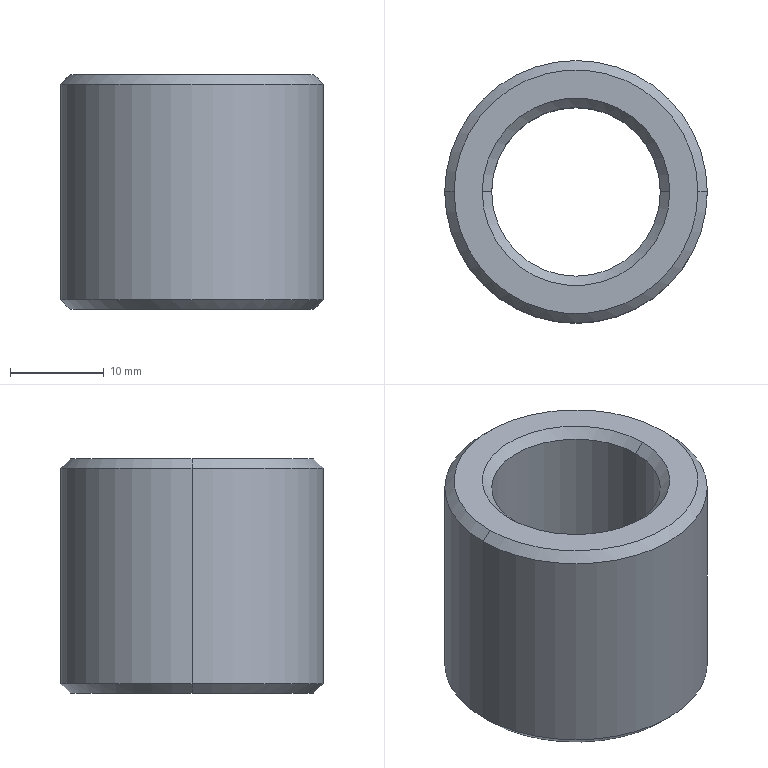Part | STEP file | VD-SYL0380DJ1006_1_2_1-9_2_STEP | 1 solid | 14 faces | box 28 x 28 x 25 mm | volume 8888 mm3 | cone 8 | cylinder 4 | plane 2 | commonest cylinder face diameters 18 x2 28 x2
STEP:
#1=CARTESIAN_POINT('',(9.,0.,-11.5));
#2=VERTEX_POINT('',#1);
#3=CARTESIAN_POINT('',(-9.,0.,-11.5));
#4=VERTEX_POINT('',#3);
#5=CARTESIAN_POINT('',(0.,0.,-11.5));
#6=DIRECTION('',(0.,0.,1.));
#7=DIRECTION('',(1.,0.,0.));
#8=AXIS2_PLACEMENT_3D('',#5,#6,#7);
#9=CIRCLE('',#8,9.);
#10=EDGE_CURVE('',#2,#4,#9,.T.);
#11=ORIENTED_EDGE('',*,*,#10,.F.);
#12=CARTESIAN_POINT('',(9.,0.,11.5));
#13=VERTEX_POINT('',#12);
#14=CARTESIAN_POINT('',(9.,0.,11.5));
#15=DIRECTION('',(0.,0.,-1.));
#16=VECTOR('',#15,1000.);
#17=LINE('',#14,#16);
#18=EDGE_CURVE('',#13,#2,#17,.T.);
#19=ORIENTED_EDGE('',*,*,#18,.F.);
#20=CARTESIAN_POINT('',(-9.,0.,11.5));
#21=VERTEX_POINT('',#20);
#22=CARTESIAN_POINT('',(0.,0.,11.5));
#23=DIRECTION('',(0.,0.,-1.));
#24=DIRECTION('',(-1.,0.,0.));
#25=AXIS2_PLACEMENT_3D('',#22,#23,#24);
#26=CIRCLE('',#25,9.);
#27=EDGE_CURVE('',#21,#13,#26,.T.);
#28=ORIENTED_EDGE('',*,*,#27,.F.);
#29=CARTESIAN_POINT('',(-9.,0.,11.5));
#30=DIRECTION('',(0.,0.,-1.));
#31=VECTOR('',#30,1000.);
#32=LINE('',#29,#31);
#33=EDGE_CURVE('',#21,#4,#32,.T.);
#34=ORIENTED_EDGE('',*,*,#33,.T.);
#35=EDGE_LOOP('',(#11,#19,#28,#34));
#36=FACE_OUTER_BOUND('',#35,.T.);
#37=CARTESIAN_POINT('',(0.,0.,-12.5));
#38=DIRECTION('',(0.,0.,1.));
#39=DIRECTION('',(1.,0.,0.));
#40=AXIS2_PLACEMENT_3D('',#37,#38,#39);
#41=CYLINDRICAL_SURFACE('',#40,9.);
#42=ADVANCED_FACE('',(#36),#41,.F.);
#43=ORIENTED_EDGE('',*,*,#27,.T.);
#44=CARTESIAN_POINT('',(10.,0.,12.5));
#45=VERTEX_POINT('',#44);
#46=CARTESIAN_POINT('',(10.,0.,12.5));
#47=DIRECTION('',(-0.7071,0.,-0.7071));
#48=VECTOR('',#47,1000.);
#49=LINE('',#46,#48);
#50=EDGE_CURVE('',#45,#13,#49,.T.);
#51=ORIENTED_EDGE('',*,*,#50,.F.);
#52=CARTESIAN_POINT('',(-10.,0.,12.5));
#53=VERTEX_POINT('',#52);
#54=CARTESIAN_POINT('',(0.,0.,12.5));
#55=DIRECTION('',(0.,0.,-1.));
#56=DIRECTION('',(-1.,0.,0.));
#57=AXIS2_PLACEMENT_3D('',#54,#55,#56);
#58=CIRCLE('',#57,10.);
#59=EDGE_CURVE('',#53,#45,#58,.T.);
#60=ORIENTED_EDGE('',*,*,#59,.F.);
#61=CARTESIAN_POINT('',(-10.,0.,12.5));
#62=DIRECTION('',(0.7071,0.,-0.7071));
#63=VECTOR('',#62,1000.);
#64=LINE('',#61,#63);
#65=EDGE_CURVE('',#53,#21,#64,.T.);
#66=ORIENTED_EDGE('',*,*,#65,.T.);
#67=EDGE_LOOP('',(#43,#51,#60,#66));
#68=FACE_OUTER_BOUND('',#67,.T.);
#69=CARTESIAN_POINT('',(0.,0.,12.));
#70=DIRECTION('',(0.,0.,1.));
#71=DIRECTION('',(1.,0.,0.));
#72=AXIS2_PLACEMENT_3D('',#69,#70,#71);
#73=CONICAL_SURFACE('',#72,9.5,0.7854);
#74=ADVANCED_FACE('',(#68),#73,.F.);
#75=ORIENTED_EDGE('',*,*,#65,.F.);
#76=CARTESIAN_POINT('',(0.,0.,12.5));
#77=DIRECTION('',(0.,0.,-1.));
#78=DIRECTION('',(1.,0.,0.));
#79=AXIS2_PLACEMENT_3D('',#76,#77,#78);
#80=CIRCLE('',#79,10.);
#81=EDGE_CURVE('',#45,#53,#80,.T.);
#82=ORIENTED_EDGE('',*,*,#81,.F.);
#83=ORIENTED_EDGE('',*,*,#50,.T.);
#84=CARTESIAN_POINT('',(0.,0.,11.5));
#85=DIRECTION('',(0.,0.,-1.));
#86=DIRECTION('',(1.,0.,0.));
#87=AXIS2_PLACEMENT_3D('',#84,#85,#86);
#88=CIRCLE('',#87,9.);
#89=EDGE_CURVE('',#13,#21,#88,.T.);
#90=ORIENTED_EDGE('',*,*,#89,.T.);
#91=EDGE_LOOP('',(#75,#82,#83,#90));
#92=FACE_OUTER_BOUND('',#91,.T.);
#93=CARTESIAN_POINT('',(0.,0.,12.));
#94=DIRECTION('',(0.,0.,1.));
#95=DIRECTION('',(1.,0.,0.));
#96=AXIS2_PLACEMENT_3D('',#93,#94,#95);
#97=CONICAL_SURFACE('',#96,9.5,0.7854);
#98=ADVANCED_FACE('',(#92),#97,.F.);
#99=CARTESIAN_POINT('',(-13.,0.,12.5));
#100=VERTEX_POINT('',#99);
#101=CARTESIAN_POINT('',(13.,0.,12.5));
#102=VERTEX_POINT('',#101);
#103=CARTESIAN_POINT('',(0.,0.,12.5));
#104=DIRECTION('',(0.,0.,1.));
#105=DIRECTION('',(-1.,0.,0.));
#106=AXIS2_PLACEMENT_3D('',#103,#104,#105);
#107=CIRCLE('',#106,13.);
#108=EDGE_CURVE('',#100,#102,#107,.T.);
#109=ORIENTED_EDGE('',*,*,#108,.F.);
#110=CARTESIAN_POINT('',(-14.,0.,11.5));
#111=VERTEX_POINT('',#110);
#112=CARTESIAN_POINT('',(-14.,0.,11.5));
#113=DIRECTION('',(0.7071,0.,0.7071));
#114=VECTOR('',#113,1000.);
#115=LINE('',#112,#114);
#116=EDGE_CURVE('',#111,#100,#115,.T.);
#117=ORIENTED_EDGE('',*,*,#116,.F.);
#118=CARTESIAN_POINT('',(14.,0.,11.5));
#119=VERTEX_POINT('',#118);
#120=CARTESIAN_POINT('',(0.,0.,11.5));
#121=DIRECTION('',(0.,0.,1.));
#122=DIRECTION('',(-1.,0.,0.));
#123=AXIS2_PLACEMENT_3D('',#120,#121,#122);
#124=CIRCLE('',#123,14.);
#125=EDGE_CURVE('',#111,#119,#124,.T.);
#126=ORIENTED_EDGE('',*,*,#125,.T.);
#127=CARTESIAN_POINT('',(14.,0.,11.5));
#128=DIRECTION('',(-0.7071,0.,0.7071));
#129=VECTOR('',#128,1000.);
#130=LINE('',#127,#129);
#131=EDGE_CURVE('',#119,#102,#130,.T.);
#132=ORIENTED_EDGE('',*,*,#131,.T.);
#133=EDGE_LOOP('',(#109,#117,#126,#132));
#134=FACE_OUTER_BOUND('',#133,.T.);
#135=CARTESIAN_POINT('',(0.,0.,12.));
#136=DIRECTION('',(0.,0.,-1.));
#137=DIRECTION('',(-1.,0.,0.));
#138=AXIS2_PLACEMENT_3D('',#135,#136,#137);
#139=CONICAL_SURFACE('',#138,13.5,0.7854);
#140=ADVANCED_FACE('',(#134),#139,.T.);
#141=ORIENTED_EDGE('',*,*,#59,.T.);
#142=ORIENTED_EDGE('',*,*,#81,.T.);
#143=EDGE_LOOP('',(#141,#142));
#144=FACE_BOUND('',#143,.T.);
#145=ORIENTED_EDGE('',*,*,#108,.T.);
#146=CARTESIAN_POINT('',(0.,0.,12.5));
#147=DIRECTION('',(0.,0.,1.));
#148=DIRECTION('',(1.,0.,0.));
#149=AXIS2_PLACEMENT_3D('',#146,#147,#148);
#150=CIRCLE('',#149,13.);
#151=EDGE_CURVE('',#102,#100,#150,.T.);
#152=ORIENTED_EDGE('',*,*,#151,.T.);
#153=EDGE_LOOP('',(#145,#152));
#154=FACE_OUTER_BOUND('',#153,.T.);
#155=CARTESIAN_POINT('',(0.,0.,12.5));
#156=DIRECTION('',(0.,0.,1.));
#157=DIRECTION('',(1.,0.,0.));
#158=AXIS2_PLACEMENT_3D('',#155,#156,#157);
#159=PLANE('',#158);
#160=ADVANCED_FACE('',(#144,#154),#159,.T.);
#161=ORIENTED_EDGE('',*,*,#131,.F.);
#162=CARTESIAN_POINT('',(0.,0.,11.5));
#163=DIRECTION('',(0.,0.,1.));
#164=DIRECTION('',(1.,0.,0.));
#165=AXIS2_PLACEMENT_3D('',#162,#163,#164);
#166=CIRCLE('',#165,14.);
#167=EDGE_CURVE('',#119,#111,#166,.T.);
#168=ORIENTED_EDGE('',*,*,#167,.T.);
#169=ORIENTED_EDGE('',*,*,#116,.T.);
#170=ORIENTED_EDGE('',*,*,#151,.F.);
#171=EDGE_LOOP('',(#161,#168,#169,#170));
#172=FACE_OUTER_BOUND('',#171,.T.);
#173=CARTESIAN_POINT('',(0.,0.,12.));
#174=DIRECTION('',(0.,0.,-1.));
#175=DIRECTION('',(-1.,0.,0.));
#176=AXIS2_PLACEMENT_3D('',#173,#174,#175);
#177=CONICAL_SURFACE('',#176,13.5,0.7854);
#178=ADVANCED_FACE('',(#172),#177,.T.);
#179=CARTESIAN_POINT('',(-14.,0.,-11.5));
#180=VERTEX_POINT('',#179);
#181=CARTESIAN_POINT('',(-14.,0.,11.5));
#182=DIRECTION('',(0.,0.,-1.));
#183=VECTOR('',#182,1000.);
#184=LINE('',#181,#183);
#185=EDGE_CURVE('',#111,#180,#184,.T.);
#186=ORIENTED_EDGE('',*,*,#185,.F.);
#187=ORIENTED_EDGE('',*,*,#167,.F.);
#188=CARTESIAN_POINT('',(14.,0.,-11.5));
#189=VERTEX_POINT('',#188);
#190=CARTESIAN_POINT('',(14.,0.,11.5));
#191=DIRECTION('',(0.,0.,-1.));
#192=VECTOR('',#191,1000.);
#193=LINE('',#190,#192);
#194=EDGE_CURVE('',#119,#189,#193,.T.);
#195=ORIENTED_EDGE('',*,*,#194,.T.);
#196=CARTESIAN_POINT('',(0.,0.,-11.5));
#197=DIRECTION('',(0.,0.,-1.));
#198=DIRECTION('',(-1.,0.,0.));
#199=AXIS2_PLACEMENT_3D('',#196,#197,#198);
#200=CIRCLE('',#199,14.);
#201=EDGE_CURVE('',#180,#189,#200,.T.);
#202=ORIENTED_EDGE('',*,*,#201,.F.);
#203=EDGE_LOOP('',(#186,#187,#195,#202));
#204=FACE_OUTER_BOUND('',#203,.T.);
#205=CARTESIAN_POINT('',(0.,0.,-12.5));
#206=DIRECTION('',(0.,0.,1.));
#207=DIRECTION('',(1.,0.,0.));
#208=AXIS2_PLACEMENT_3D('',#205,#206,#207);
#209=CYLINDRICAL_SURFACE('',#208,14.);
#210=ADVANCED_FACE('',(#204),#209,.T.);
#211=CARTESIAN_POINT('',(0.,0.,-11.5));
#212=DIRECTION('',(0.,0.,-1.));
#213=DIRECTION('',(1.,0.,0.));
#214=AXIS2_PLACEMENT_3D('',#211,#212,#213);
#215=CIRCLE('',#214,14.);
#216=EDGE_CURVE('',#189,#180,#215,.T.);
#217=ORIENTED_EDGE('',*,*,#216,.F.);
#218=ORIENTED_EDGE('',*,*,#194,.F.);
#219=ORIENTED_EDGE('',*,*,#125,.F.);
#220=ORIENTED_EDGE('',*,*,#185,.T.);
#221=EDGE_LOOP('',(#217,#218,#219,#220));
#222=FACE_OUTER_BOUND('',#221,.T.);
#223=CARTESIAN_POINT('',(0.,0.,-12.5));
#224=DIRECTION('',(0.,0.,1.));
#225=DIRECTION('',(1.,0.,0.));
#226=AXIS2_PLACEMENT_3D('',#223,#224,#225);
#227=CYLINDRICAL_SURFACE('',#226,14.);
#228=ADVANCED_FACE('',(#222),#227,.T.);
#229=CARTESIAN_POINT('',(13.,0.,-12.5));
#230=VERTEX_POINT('',#229);
#231=CARTESIAN_POINT('',(-13.,0.,-12.5));
#232=VERTEX_POINT('',#231);
#233=CARTESIAN_POINT('',(0.,0.,-12.5));
#234=DIRECTION('',(0.,0.,-1.));
#235=DIRECTION('',(1.,0.,0.));
#236=AXIS2_PLACEMENT_3D('',#233,#234,#235);
#237=CIRCLE('',#236,13.);
#238=EDGE_CURVE('',#230,#232,#237,.T.);
#239=ORIENTED_EDGE('',*,*,#238,.F.);
#240=CARTESIAN_POINT('',(14.,0.,-11.5));
#241=DIRECTION('',(-0.7071,0.,-0.7071));
#242=VECTOR('',#241,1000.);
#243=LINE('',#240,#242);
#244=EDGE_CURVE('',#189,#230,#243,.T.);
#245=ORIENTED_EDGE('',*,*,#244,.F.);
#246=ORIENTED_EDGE('',*,*,#216,.T.);
#247=CARTESIAN_POINT('',(-14.,0.,-11.5));
#248=DIRECTION('',(0.7071,0.,-0.7071));
#249=VECTOR('',#248,1000.);
#250=LINE('',#247,#249);
#251=EDGE_CURVE('',#180,#232,#250,.T.);
#252=ORIENTED_EDGE('',*,*,#251,.T.);
#253=EDGE_LOOP('',(#239,#245,#246,#252));
#254=FACE_OUTER_BOUND('',#253,.T.);
#255=CARTESIAN_POINT('',(0.,0.,-12.));
#256=DIRECTION('',(0.,0.,1.));
#257=DIRECTION('',(1.,0.,0.));
#258=AXIS2_PLACEMENT_3D('',#255,#256,#257);
#259=CONICAL_SURFACE('',#258,13.5,0.7854);
#260=ADVANCED_FACE('',(#254),#259,.T.);
#261=ORIENTED_EDGE('',*,*,#251,.F.);
#262=ORIENTED_EDGE('',*,*,#201,.T.);
#263=ORIENTED_EDGE('',*,*,#244,.T.);
#264=CARTESIAN_POINT('',(0.,0.,-12.5));
#265=DIRECTION('',(0.,0.,-1.));
#266=DIRECTION('',(-1.,0.,0.));
#267=AXIS2_PLACEMENT_3D('',#264,#265,#266);
#268=CIRCLE('',#267,13.);
#269=EDGE_CURVE('',#232,#230,#268,.T.);
#270=ORIENTED_EDGE('',*,*,#269,.F.);
#271=EDGE_LOOP('',(#261,#262,#263,#270));
#272=FACE_OUTER_BOUND('',#271,.T.);
#273=CARTESIAN_POINT('',(0.,0.,-12.));
#274=DIRECTION('',(0.,0.,1.));
#275=DIRECTION('',(1.,0.,0.));
#276=AXIS2_PLACEMENT_3D('',#273,#274,#275);
#277=CONICAL_SURFACE('',#276,13.5,0.7854);
#278=ADVANCED_FACE('',(#272),#277,.T.);
#279=CARTESIAN_POINT('',(-10.,0.,-12.5));
#280=VERTEX_POINT('',#279);
#281=CARTESIAN_POINT('',(10.,0.,-12.5));
#282=VERTEX_POINT('',#281);
#283=CARTESIAN_POINT('',(0.,0.,-12.5));
#284=DIRECTION('',(0.,0.,1.));
#285=DIRECTION('',(-1.,0.,0.));
#286=AXIS2_PLACEMENT_3D('',#283,#284,#285);
#287=CIRCLE('',#286,10.);
#288=EDGE_CURVE('',#280,#282,#287,.T.);
#289=ORIENTED_EDGE('',*,*,#288,.T.);
#290=CARTESIAN_POINT('',(0.,0.,-12.5));
#291=DIRECTION('',(0.,0.,1.));
#292=DIRECTION('',(1.,0.,0.));
#293=AXIS2_PLACEMENT_3D('',#290,#291,#292);
#294=CIRCLE('',#293,10.);
#295=EDGE_CURVE('',#282,#280,#294,.T.);
#296=ORIENTED_EDGE('',*,*,#295,.T.);
#297=EDGE_LOOP('',(#289,#296));
#298=FACE_BOUND('',#297,.T.);
#299=ORIENTED_EDGE('',*,*,#238,.T.);
#300=ORIENTED_EDGE('',*,*,#269,.T.);
#301=EDGE_LOOP('',(#299,#300));
#302=FACE_OUTER_BOUND('',#301,.T.);
#303=CARTESIAN_POINT('',(0.,0.,-12.5));
#304=DIRECTION('',(0.,0.,1.));
#305=DIRECTION('',(1.,0.,0.));
#306=AXIS2_PLACEMENT_3D('',#303,#304,#305);
#307=PLANE('',#306);
#308=ADVANCED_FACE('',(#298,#302),#307,.F.);
#309=ORIENTED_EDGE('',*,*,#10,.T.);
#310=CARTESIAN_POINT('',(-10.,0.,-12.5));
#311=DIRECTION('',(0.7071,0.,0.7071));
#312=VECTOR('',#311,1000.);
#313=LINE('',#310,#312);
#314=EDGE_CURVE('',#280,#4,#313,.T.);
#315=ORIENTED_EDGE('',*,*,#314,.F.);
#316=ORIENTED_EDGE('',*,*,#295,.F.);
#317=CARTESIAN_POINT('',(10.,0.,-12.5));
#318=DIRECTION('',(-0.7071,0.,0.7071));
#319=VECTOR('',#318,1000.);
#320=LINE('',#317,#319);
#321=EDGE_CURVE('',#282,#2,#320,.T.);
#322=ORIENTED_EDGE('',*,*,#321,.T.);
#323=EDGE_LOOP('',(#309,#315,#316,#322));
#324=FACE_OUTER_BOUND('',#323,.T.);
#325=CARTESIAN_POINT('',(0.,0.,-12.));
#326=DIRECTION('',(0.,0.,-1.));
#327=DIRECTION('',(-1.,0.,0.));
#328=AXIS2_PLACEMENT_3D('',#325,#326,#327);
#329=CONICAL_SURFACE('',#328,9.5,0.7854);
#330=ADVANCED_FACE('',(#324),#329,.F.);
#331=ORIENTED_EDGE('',*,*,#321,.F.);
#332=ORIENTED_EDGE('',*,*,#288,.F.);
#333=ORIENTED_EDGE('',*,*,#314,.T.);
#334=CARTESIAN_POINT('',(0.,0.,-11.5));
#335=DIRECTION('',(0.,0.,1.));
#336=DIRECTION('',(-1.,0.,0.));
#337=AXIS2_PLACEMENT_3D('',#334,#335,#336);
#338=CIRCLE('',#337,9.);
#339=EDGE_CURVE('',#4,#2,#338,.T.);
#340=ORIENTED_EDGE('',*,*,#339,.T.);
#341=EDGE_LOOP('',(#331,#332,#333,#340));
#342=FACE_OUTER_BOUND('',#341,.T.);
#343=CARTESIAN_POINT('',(0.,0.,-12.));
#344=DIRECTION('',(0.,0.,-1.));
#345=DIRECTION('',(-1.,0.,0.));
#346=AXIS2_PLACEMENT_3D('',#343,#344,#345);
#347=CONICAL_SURFACE('',#346,9.5,0.7854);
#348=ADVANCED_FACE('',(#342),#347,.F.);
#349=ORIENTED_EDGE('',*,*,#33,.F.);
#350=ORIENTED_EDGE('',*,*,#89,.F.);
#351=ORIENTED_EDGE('',*,*,#18,.T.);
#352=ORIENTED_EDGE('',*,*,#339,.F.);
#353=EDGE_LOOP('',(#349,#350,#351,#352));
#354=FACE_OUTER_BOUND('',#353,.T.);
#355=CARTESIAN_POINT('',(0.,0.,-12.5));
#356=DIRECTION('',(0.,0.,1.));
#357=DIRECTION('',(1.,0.,0.));
#358=AXIS2_PLACEMENT_3D('',#355,#356,#357);
#359=CYLINDRICAL_SURFACE('',#358,9.);
#360=ADVANCED_FACE('',(#354),#359,.F.);
#361=CLOSED_SHELL('',(#42,#74,#98,#140,#160,#178,#210,#228,#260,#278,#308,#330,#348,#360));
#362=MANIFOLD_SOLID_BREP('',#361);
#363=CARTESIAN_POINT('',(0.,0.,0.));
#364=DIRECTION('',(0.,0.,1.));
#365=DIRECTION('',(1.,0.,0.));
#366=AXIS2_PLACEMENT_3D('',#363,#364,#365);
#367=(LENGTH_UNIT()NAMED_UNIT(*)SI_UNIT(.MILLI.,.METRE.));
#368=UNCERTAINTY_MEASURE_WITH_UNIT(LENGTH_MEASURE(0.00001),#367,'','');
#369=(NAMED_UNIT(*)PLANE_ANGLE_UNIT()SI_UNIT($,.RADIAN.));
#370=(NAMED_UNIT(*)SI_UNIT($,.STERADIAN.)SOLID_ANGLE_UNIT());
#371=(GEOMETRIC_REPRESENTATION_CONTEXT(3)GLOBAL_UNCERTAINTY_ASSIGNED_CONTEXT((#368))GLOBAL_UNIT_ASSIGNED_CONTEXT((#367,#369,#370))REPRESENTATION_CONTEXT('',''));
#372=ADVANCED_BREP_SHAPE_REPRESENTATION('',(#362,#366),#371);